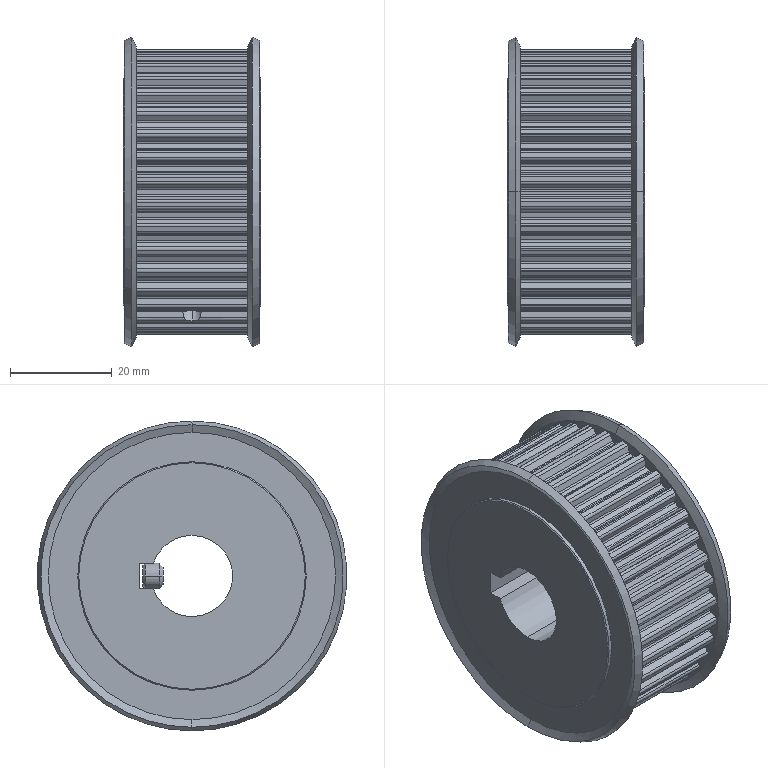Part | SolidWorks | 3 solids | 410 faces | box 27 x 61 x 61 mm | volume 57710 mm3 | cylinder 271 | plane 113 | cone 26 | commonest cylinder face diameters 0.8 x91 1.2 x90 52.85 x39 56.45 x36 4.134 x4 5 x4